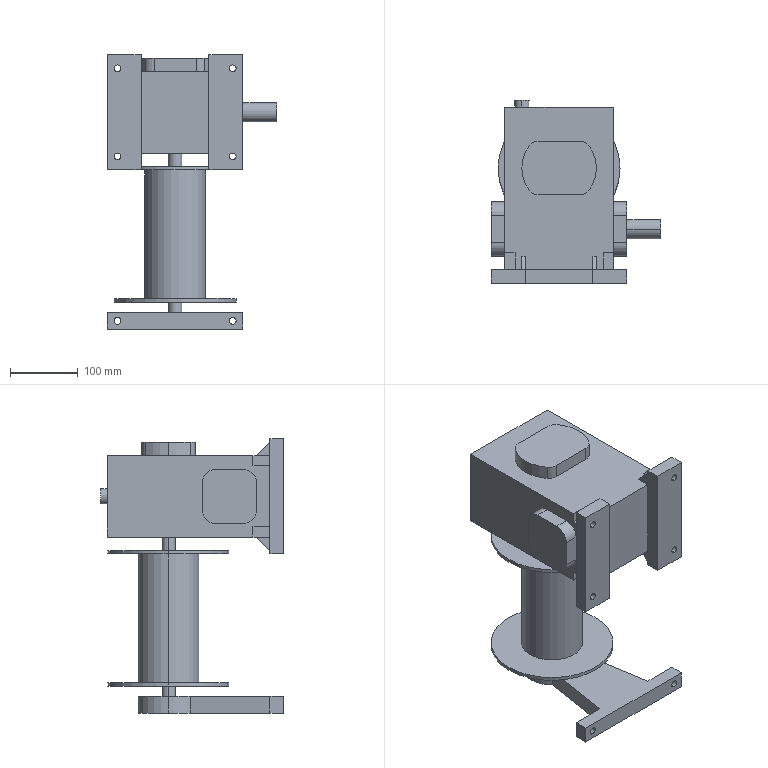Part | SolidWorks | features ICE 11, Fillet 2, MirrorPattern 1, Revolution 1 | 3 solids | 115 faces | box 250 x 270 x 405 mm | volume 7312574 mm3 | plane 69 | cylinder 46 | commonest cylinder face diameters 10 x12 40 x8 20 x6 90 x5 32 x4 180 x4